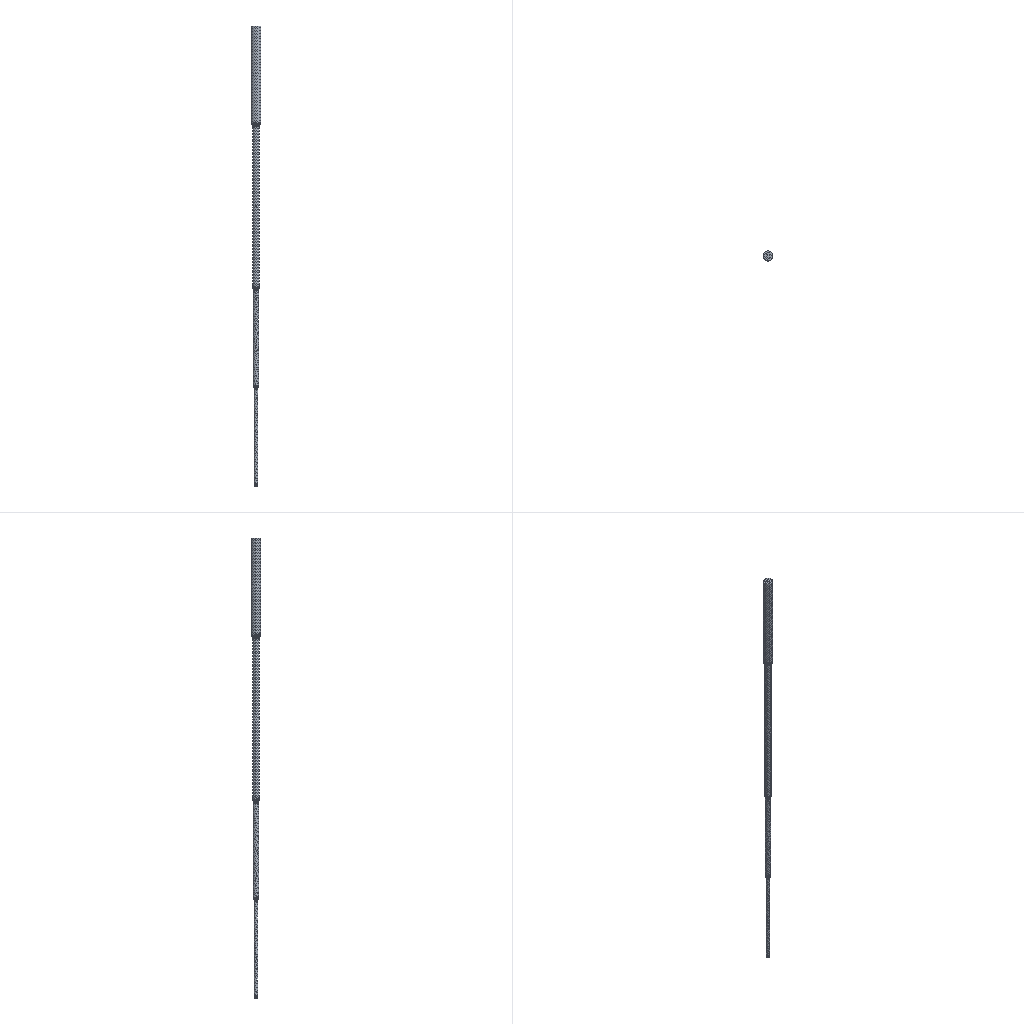Simulation study | ansys workbench
Set-up summary:
category,name,step,type,value,unit,region
solver,ansys_workbench
units,mm-N-s-tonne (MPa),,stated,"/units,MPA"
analysis,LS1,,static
load_step,LS1,LS1,static,nsubst=1; time=1
mesh,nodes,,,72464
mesh,elements,,,46318
element_type,SOLID187,,,46255
element_type,SURF154,,,63
material,Structural Steel,,E,200000,tonne s^-2 mm^-1
material,Structural Steel,,nu,0.3
material,Structural Steel,,density,7.85e-09,tonne mm^-3
material,Structural Steel,,conductivity,60.5,tonne mm s^-3 C^-1
material,Structural Steel,,specific_heat,4.34e+08,mm^2 s^-2 C^-1
material,Structural Steel,,cte,1.2e-05,C^-1
material,Structural Steel,,permeability,10000
material,Structural Steel,,resistivity,0.00017,ohm mm
load,Define Force Using Surface Effect Elements,LS1,surface-effect pres face 1,1.273,,SURF154 #2
load,Define Force Using Surface Effect Elements,LS1,surface-effect pres face 3,1.273,,SURF154 #2
bc,Fixed Supports,model,fixed,[dofs=ALL],,_FIXEDSU
named_set,_FIXEDSU,,node,6080
Ansys APDL input file, long lists of numbers shortened:
/batch
/config,noeldb,1     ! force off writing results to database
*get,_wallstrt,active,,time,wall
! ANSYS input file written by Workbench version 2023 R1
! File used for geometry attach:
/title,E1.7.1--Static Structural (A5)
! ****** Begin Custom Load Command Snippet ******
/COM, ACT Extensions:
/COM,     LSDYNA, 2023.1
/COM,/COM,     ANSYSMotion, 2023.1
/COM,
! ****** End   Custom Load Command Snippet ******
*DIM,_wb_ProjectScratch_dir,string,248
_wb_ProjectScratch_dir(1) = ''
*DIM,_wb_SolverFiles_dir,string,248
_wb_SolverFiles_dir(1) = ''
*DIM,_wb_userfiles_dir,string,248
_wb_userfiles_dir(1) = ''
/com,--- Data in consistent NMM units. See Solving Units in the help system for more information.
/units,MPA
/nopr
/wb,file,start              !  signify a WB generated input file
/prep7
! Turn off shape checking because checks already performed inside WB mesher.
! See help system for more information.
SHPP,OFF,,NOWARN
/nolist
etcon,set             ! allow ANSYS to choose best KEYOP's for 180x elements, resets any applicable keyopt to MAPDL defaults
/com,*********** Nodes for the whole assembly ***********
nblock,3,,79710
(1i9,3e20.9e3)
        1     1.438136494E+00     2.540091588E+00     9.554998962E-01
! (72463 more lines like these left out)
-1
/wb,elem,start            !  set before creation of elements
/com,*********** Elements for Body 1 "1" ***********
et,1,187
eblock,19,solid,,46255
(19i9)
        1        1        1        1        0        0        0        0       10        0        1     3322     3325     3311     3308    12482    11804    10592    10591
! (92509 more lines like these left out)
-1
/wb,elem,end               !  done creating elements
/com,*********** Send User Defined Coordinate System(s) ***********
csys,0
toffst,273.15,  ! Temperature offset from absolute zero
/com,*********** Set Reference Temperature ***********
tref,22.
/wb,mat,start              !  starting to send materials
/com,*********** Send Materials ***********
Temperature = 'TEMP' ! Temperature
MP,DENS,1,7.85e-09,	! tonne mm^-3
MP,ALPX,1,1.2e-05,	! C^-1
MP,C,1,434000000,	! mm^2 s^-2 C^-1
MP,KXX,1,60.5,	! tonne mm s^-3 C^-1
MP,RSVX,1,0.00017,	! ohm mm
MP,EX,1,200000,	! tonne s^-2 mm^-1
MP,NUXY,1,0.3,
MP,MURX,1,10000,
/wb,mat,end                !  done sending materials
!************************* Model Summary ********************
!1,	Structural Steel,	matid,	1
!************************* End Model Summary ********************
! get the diagonal of the bounding box. Needed later for other things
*get,_xmin,node,,mnloc,x
*get,_ymin,node,,mnloc,y
*get,_zmin,node,,mnloc,z
*get,_xmax,node,,mxloc,x
*get,_ymax,node,,mxloc,y
*get,_zmax,node,,mxloc,z
_ASMDIAG=(_xmax-_xmin)*(_xmax-_xmin)+(_ymax-_ymin)*(_ymax-_ymin)+(_zmax-_zmin)*(_zmax-_zmin)
_ASMDIAG=SQRT(_ASMDIAG)
/wb,contact,start          !  starting to send contact
/wb,contact,end            !  done creating contacts
/golist
/wb,load,start             !  starting to send loads
/com,*********** Fixed Supports ***********
CMBLOCK,_FIXEDSU,NODE,     6080
(8i10)
       179       180       181       182       184       185       186       188
! (759 more lines like these left out)
cmsel,s,_FIXEDSU
d,all,all
nsel,all
/com,*********** Define Force Using Surface Effect Elements ***********
local,12,0,0.,0.,0.,0.,0.,0.
csys,0
et,2,154
mat,2
eblock,10,,,63
(15i9)
    56316        2        2        2       12    10583      551      545      545    26951    26992      545    26991
! (62 more lines like these left out)
-1
esel,s,type,,2
keyop,2,2,1                ! Apply load in local coordinate system
keyop,2,7,1                ! Use original area so load is constant in large deformation
esel,all
/gst,on,on
fini
*get,_numnode,node,0,count
*get,_numelem,elem,0,count
*get, _MAXELEMNUM, elem, 0, NUM, MAX
*get, _MAXNODENUM, node, 0, NUM, MAX
*get, _MAXELEMTYPE, etyp, 0, NUM, MAX
*get, _MAXREALCONST, rcon, 0, NUM, MAX
/go
/wb,load,end               !  done creating loads
/com,--- Number of total nodes = %_numnode%
/com,--- Number of contact elements = 63
/com,--- Number of spring elements = 0
/com,--- Number of bearing elements = 0
/com,--- Number of solid elements = 46255
/com,--- Number of condensed parts = 0
/com,--- Number of total elements = %_numelem%
*get,_wallbsol,active,,time,wall
/com,****************************************************************************
/com,*************************    SOLUTION       ********************************
/com,****************************************************************************
/solu
antype,0                   ! static analysis
_thickRatio=  1     ! Ratio of thick parts in the model
eqsl,pcg,1e-8,,,,,,1
cntr,print,1               ! print out contact info and also make no initial contact an error
nldiag,cont,iter           ! print out contact info each equilibrium iteration
rescontrol,,none                 ! Do not keep any restart files
/com,****************************************************
/com,******************* SOLVE FOR LS 1 OF 1 ****************
esel,s,type,,2
nsle
sfe,all,1,pres,1,1.273
sfe,all,2,pres,1,0.
sfe,all,3,pres,1,1.273
nsel,all
esel,all
/nopr
/gopr
autots,on                   ! User turned on automatic time stepping
nsub,1,10,1,OFF
time,1.
outres,erase
outres,all,none
outres,nsol,all,
outres,rsol,all
outres,eangl,all
outres,etmp,all
outres,veng,all
outres,strs,all,
outres,epel,all,
outres,eppl,all,
outres,cont,all,
! *********** WB SOLVE COMMAND ***********
! check interactive state
*get,ANSINTER_,active,,int
*if,ANSINTER_,ne,0,then
/eof
*endif
solve
/com *************** Write FE CONNECTORS *********
CEWRITE,file,ce,,INTE
/com,****************************************************
/com,*************** FINISHED SOLVE FOR LS 1 *************
*get,_wallasol,active,,time,wall
/nopr
*get,_numnode,node,0,count
*get,_numelem,elem,0,count
*get, _MAXELEMNUM, elem, 0, NUM, MAX
*get, _MAXNODENUM, node, 0, NUM, MAX,,,INTERNAL
*get, _MAXELEMTYPE, etyp, 0, NUM, MAX
*get, _MAXREALCONST, rcon, 0, NUM, MAX
*get,_NSOLTHREADS,active,0,ntfs
*get,_NSOLPROCESSES,active,0,npfs
/gopr
*get,_PCGITER,active,,solu,cgiter
/post1
xmlo,ENCODING,ISO-8859-1
xmlo,parm
/xml,parm,xml
fini
/gopr
*get,_walldone,active,,time,wall
_preptime=(_wallbsol-_wallstrt)*3600
_solvtime=(_wallasol-_wallbsol)*3600
_posttime=(_walldone-_wallasol)*3600
_totaltim=(_walldone-_wallstrt)*3600
*get,_dlbratio,active,0,solu,dlbr
*get,_combtime,active,0,solu,comb
*get,_ssmode,active,0,solu,ssmm
*get,_ndofs,active,0,solu,ndof
/com,--- Total number of nodes = %_numnode%
/com,--- Total number of elements = %_numelem%
/com,--- Element load balance ratio = %_dlbratio%
/com,--- Time to combine distributed files = %_combtime%
/com,--- Sparse memory mode = %_ssmode%
/com,--- Number of DOF = %_ndofs%
/wb,file,end               ! done with WB generated input
Results summary:
result,analyses[0].index,,,1
result,analyses[0].system,,,SYS
result,analyses[0].deck,,,deck.dat
result,analyses[0].solve_status,,,completed
result,analyses[0].analysis_type,,,static
result,analyses[0].physics,,,mechanical
result,analyses[0].unit_system,,,"NMM: mm, ton, N, s, mV, mA, degC"
result,analyses[0].n_sets,,,1
result,analyses[0].load_steps[0].set,set=1,,1
result,analyses[0].load_steps[0].time_or_freq,set=1,,1
result,analyses[0].load_steps[0].max_displacement_magnitude,set=1,,43.269
result,analyses[0].load_steps[0].max_von_mises_nodal,set=1,,308.352
result,analyses[0].load_steps[0].reaction_force_sum_xyz[1],set=1,,-100
result,analyses[0].load_steps[0].reaction_force_sum_xyz[2],set=1,,-6.32692e-06
result,analyses[0].load_steps[0].reaction_force_sum_xyz[3],set=1,,-100
result,geometry_export[0][0],,,.step
result,geometry_export[0][1],,,ok
result,geometry_export[0][2],,,1